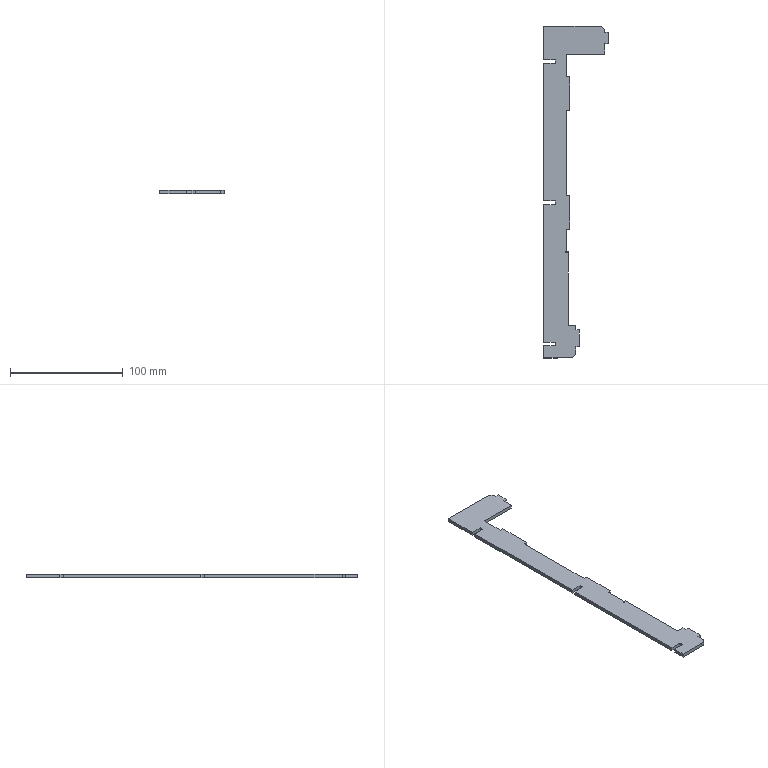Part | SolidWorks | features FlatPattern 1, SMBaseFlange 1, SheetMetal 1 | 1 solid | 46 faces | box 57 x 294.081 x 3.2 mm | volume 23149 mm3 | plane 40 | cylinder 6 | commonest cylinder face diameters 1 x2 1.5 x2 10 x2
STEP:
#1=CARTESIAN_POINT('',(397.65,-115.276,3.2));
#2=VERTEX_POINT('',#1);
#3=CARTESIAN_POINT('',(398.1,-114.588,3.2));
#4=VERTEX_POINT('',#3);
#5=CARTESIAN_POINT('',(398.4,-115.276,3.2));
#6=DIRECTION('',(0.,0.,-1.));
#7=DIRECTION('',(1.,0.,0.));
#8=AXIS2_PLACEMENT_3D('',#5,#6,#7);
#9=CIRCLE('',#8,0.75);
#10=EDGE_CURVE('',#2,#4,#9,.T.);
#11=ORIENTED_EDGE('',*,*,#10,.F.);
#12=CARTESIAN_POINT('',(397.65,-115.276,0.));
#13=VERTEX_POINT('',#12);
#14=CARTESIAN_POINT('',(397.65,-115.276,3.2));
#15=DIRECTION('',(0.,0.,-1.));
#16=VECTOR('',#15,1000.);
#17=LINE('',#14,#16);
#18=EDGE_CURVE('',#2,#13,#17,.T.);
#19=ORIENTED_EDGE('',*,*,#18,.T.);
#20=CARTESIAN_POINT('',(398.1,-114.588,0.));
#21=VERTEX_POINT('',#20);
#22=CARTESIAN_POINT('',(398.4,-115.276,0.));
#23=DIRECTION('',(0.,0.,-1.));
#24=DIRECTION('',(1.,0.,0.));
#25=AXIS2_PLACEMENT_3D('',#22,#23,#24);
#26=CIRCLE('',#25,0.75);
#27=EDGE_CURVE('',#13,#21,#26,.T.);
#28=ORIENTED_EDGE('',*,*,#27,.T.);
#29=CARTESIAN_POINT('',(398.1,-114.588,3.2));
#30=DIRECTION('',(0.,0.,-1.));
#31=VECTOR('',#30,1000.);
#32=LINE('',#29,#31);
#33=EDGE_CURVE('',#4,#21,#32,.T.);
#34=ORIENTED_EDGE('',*,*,#33,.F.);
#35=EDGE_LOOP('',(#11,#19,#28,#34));
#36=FACE_OUTER_BOUND('',#35,.T.);
#37=CARTESIAN_POINT('',(398.4,-115.276,3.2));
#38=DIRECTION('',(0.,0.,-1.));
#39=DIRECTION('',(-1.,0.,0.));
#40=AXIS2_PLACEMENT_3D('',#37,#38,#39);
#41=CYLINDRICAL_SURFACE('',#40,0.75);
#42=ADVANCED_FACE('',(#36),#41,.F.);
#43=CARTESIAN_POINT('',(432.4,59.724,0.));
#44=VERTEX_POINT('',#43);
#45=CARTESIAN_POINT('',(432.4,69.224,0.));
#46=VERTEX_POINT('',#45);
#47=CARTESIAN_POINT('',(432.4,59.724,0.));
#48=DIRECTION('',(0.,1.,0.));
#49=VECTOR('',#48,1000.);
#50=LINE('',#47,#49);
#51=EDGE_CURVE('',#44,#46,#50,.T.);
#52=ORIENTED_EDGE('',*,*,#51,.T.);
#53=CARTESIAN_POINT('',(432.4,69.224,3.2));
#54=VERTEX_POINT('',#53);
#55=CARTESIAN_POINT('',(432.4,69.224,3.2));
#56=DIRECTION('',(0.,0.,-1.));
#57=VECTOR('',#56,1000.);
#58=LINE('',#55,#57);
#59=EDGE_CURVE('',#54,#46,#58,.T.);
#60=ORIENTED_EDGE('',*,*,#59,.F.);
#61=CARTESIAN_POINT('',(432.4,59.724,3.2));
#62=VERTEX_POINT('',#61);
#63=CARTESIAN_POINT('',(432.4,59.724,3.2));
#64=DIRECTION('',(0.,1.,0.));
#65=VECTOR('',#64,1000.);
#66=LINE('',#63,#65);
#67=EDGE_CURVE('',#62,#54,#66,.T.);
#68=ORIENTED_EDGE('',*,*,#67,.F.);
#69=CARTESIAN_POINT('',(432.4,59.724,3.2));
#70=DIRECTION('',(0.,0.,-1.));
#71=VECTOR('',#70,1000.);
#72=LINE('',#69,#71);
#73=EDGE_CURVE('',#62,#44,#72,.T.);
#74=ORIENTED_EDGE('',*,*,#73,.T.);
#75=EDGE_LOOP('',(#52,#60,#68,#74));
#76=FACE_OUTER_BOUND('',#75,.T.);
#77=CARTESIAN_POINT('',(432.4,59.724,3.2));
#78=DIRECTION('',(-1.,0.,0.));
#79=DIRECTION('',(0.,0.,1.));
#80=AXIS2_PLACEMENT_3D('',#77,#78,#79);
#81=PLANE('',#80);
#82=ADVANCED_FACE('',(#76),#81,.F.);
#83=CARTESIAN_POINT('',(435.4,69.224,0.));
#84=VERTEX_POINT('',#83);
#85=CARTESIAN_POINT('',(435.4,69.224,0.));
#86=DIRECTION('',(1.,0.,0.));
#87=VECTOR('',#86,1000.);
#88=LINE('',#85,#87);
#89=EDGE_CURVE('',#46,#84,#88,.T.);
#90=ORIENTED_EDGE('',*,*,#89,.T.);
#91=CARTESIAN_POINT('',(435.4,69.224,3.2));
#92=VERTEX_POINT('',#91);
#93=CARTESIAN_POINT('',(435.4,69.224,3.2));
#94=DIRECTION('',(0.,0.,-1.));
#95=VECTOR('',#94,1000.);
#96=LINE('',#93,#95);
#97=EDGE_CURVE('',#92,#84,#96,.T.);
#98=ORIENTED_EDGE('',*,*,#97,.F.);
#99=CARTESIAN_POINT('',(435.4,69.224,3.2));
#100=DIRECTION('',(1.,0.,0.));
#101=VECTOR('',#100,1000.);
#102=LINE('',#99,#101);
#103=EDGE_CURVE('',#54,#92,#102,.T.);
#104=ORIENTED_EDGE('',*,*,#103,.F.);
#105=ORIENTED_EDGE('',*,*,#59,.T.);
#106=EDGE_LOOP('',(#90,#98,#104,#105));
#107=FACE_OUTER_BOUND('',#106,.T.);
#108=CARTESIAN_POINT('',(435.4,69.224,3.2));
#109=DIRECTION('',(0.,1.,0.));
#110=DIRECTION('',(0.,0.,1.));
#111=AXIS2_PLACEMENT_3D('',#108,#109,#110);
#112=PLANE('',#111);
#113=ADVANCED_FACE('',(#107),#112,.F.);
#114=CARTESIAN_POINT('',(435.4,79.224,0.));
#115=VERTEX_POINT('',#114);
#116=CARTESIAN_POINT('',(435.4,79.224,0.));
#117=DIRECTION('',(0.,1.,0.));
#118=VECTOR('',#117,1000.);
#119=LINE('',#116,#118);
#120=EDGE_CURVE('',#84,#115,#119,.T.);
#121=ORIENTED_EDGE('',*,*,#120,.T.);
#122=CARTESIAN_POINT('',(435.4,79.224,3.2));
#123=VERTEX_POINT('',#122);
#124=CARTESIAN_POINT('',(435.4,79.224,3.2));
#125=DIRECTION('',(0.,0.,-1.));
#126=VECTOR('',#125,1000.);
#127=LINE('',#124,#126);
#128=EDGE_CURVE('',#123,#115,#127,.T.);
#129=ORIENTED_EDGE('',*,*,#128,.F.);
#130=CARTESIAN_POINT('',(435.4,79.224,3.2));
#131=DIRECTION('',(0.,1.,0.));
#132=VECTOR('',#131,1000.);
#133=LINE('',#130,#132);
#134=EDGE_CURVE('',#92,#123,#133,.T.);
#135=ORIENTED_EDGE('',*,*,#134,.F.);
#136=ORIENTED_EDGE('',*,*,#97,.T.);
#137=EDGE_LOOP('',(#121,#129,#135,#136));
#138=FACE_OUTER_BOUND('',#137,.T.);
#139=CARTESIAN_POINT('',(435.4,79.224,3.2));
#140=DIRECTION('',(-1.,0.,0.));
#141=DIRECTION('',(0.,-1.,0.));
#142=AXIS2_PLACEMENT_3D('',#139,#140,#141);
#143=PLANE('',#142);
#144=ADVANCED_FACE('',(#138),#143,.F.);
#145=CARTESIAN_POINT('',(432.4,79.224,0.));
#146=VERTEX_POINT('',#145);
#147=CARTESIAN_POINT('',(432.4,79.224,0.));
#148=DIRECTION('',(-1.,0.,0.));
#149=VECTOR('',#148,1000.);
#150=LINE('',#147,#149);
#151=EDGE_CURVE('',#115,#146,#150,.T.);
#152=ORIENTED_EDGE('',*,*,#151,.T.);
#153=CARTESIAN_POINT('',(432.4,79.224,3.2));
#154=VERTEX_POINT('',#153);
#155=CARTESIAN_POINT('',(432.4,79.224,3.2));
#156=DIRECTION('',(0.,0.,-1.));
#157=VECTOR('',#156,1000.);
#158=LINE('',#155,#157);
#159=EDGE_CURVE('',#154,#146,#158,.T.);
#160=ORIENTED_EDGE('',*,*,#159,.F.);
#161=CARTESIAN_POINT('',(432.4,79.224,3.2));
#162=DIRECTION('',(-1.,0.,0.));
#163=VECTOR('',#162,1000.);
#164=LINE('',#161,#163);
#165=EDGE_CURVE('',#123,#154,#164,.T.);
#166=ORIENTED_EDGE('',*,*,#165,.F.);
#167=ORIENTED_EDGE('',*,*,#128,.T.);
#168=EDGE_LOOP('',(#152,#160,#166,#167));
#169=FACE_OUTER_BOUND('',#168,.T.);
#170=CARTESIAN_POINT('',(432.4,79.224,3.2));
#171=DIRECTION('',(0.,-1.,0.));
#172=DIRECTION('',(1.,0.,0.));
#173=AXIS2_PLACEMENT_3D('',#170,#171,#172);
#174=PLANE('',#173);
#175=ADVANCED_FACE('',(#169),#174,.F.);
#176=CARTESIAN_POINT('',(432.4,79.724,0.));
#177=VERTEX_POINT('',#176);
#178=CARTESIAN_POINT('',(432.4,79.224,0.));
#179=DIRECTION('',(0.,1.,0.));
#180=VECTOR('',#179,1000.);
#181=LINE('',#178,#180);
#182=EDGE_CURVE('',#146,#177,#181,.T.);
#183=ORIENTED_EDGE('',*,*,#182,.T.);
#184=CARTESIAN_POINT('',(432.4,79.724,3.2));
#185=VERTEX_POINT('',#184);
#186=CARTESIAN_POINT('',(432.4,79.724,3.2));
#187=DIRECTION('',(0.,0.,-1.));
#188=VECTOR('',#187,1000.);
#189=LINE('',#186,#188);
#190=EDGE_CURVE('',#185,#177,#189,.T.);
#191=ORIENTED_EDGE('',*,*,#190,.F.);
#192=CARTESIAN_POINT('',(432.4,79.224,3.2));
#193=DIRECTION('',(0.,1.,0.));
#194=VECTOR('',#193,1000.);
#195=LINE('',#192,#194);
#196=EDGE_CURVE('',#154,#185,#195,.T.);
#197=ORIENTED_EDGE('',*,*,#196,.F.);
#198=ORIENTED_EDGE('',*,*,#159,.T.);
#199=EDGE_LOOP('',(#183,#191,#197,#198));
#200=FACE_OUTER_BOUND('',#199,.T.);
#201=CARTESIAN_POINT('',(432.4,79.224,3.2));
#202=DIRECTION('',(-1.,0.,0.));
#203=DIRECTION('',(0.,0.,1.));
#204=AXIS2_PLACEMENT_3D('',#201,#202,#203);
#205=PLANE('',#204);
#206=ADVANCED_FACE('',(#200),#205,.F.);
#207=CARTESIAN_POINT('',(427.4,84.724,0.));
#208=VERTEX_POINT('',#207);
#209=CARTESIAN_POINT('',(427.4,79.724,0.));
#210=DIRECTION('',(0.,0.,1.));
#211=DIRECTION('',(-1.,0.,0.));
#212=AXIS2_PLACEMENT_3D('',#209,#210,#211);
#213=CIRCLE('',#212,5.);
#214=EDGE_CURVE('',#177,#208,#213,.T.);
#215=ORIENTED_EDGE('',*,*,#214,.T.);
#216=CARTESIAN_POINT('',(427.4,84.724,3.2));
#217=VERTEX_POINT('',#216);
#218=CARTESIAN_POINT('',(427.4,84.724,3.2));
#219=DIRECTION('',(0.,0.,-1.));
#220=VECTOR('',#219,1000.);
#221=LINE('',#218,#220);
#222=EDGE_CURVE('',#217,#208,#221,.T.);
#223=ORIENTED_EDGE('',*,*,#222,.F.);
#224=CARTESIAN_POINT('',(427.4,79.724,3.2));
#225=DIRECTION('',(0.,0.,1.));
#226=DIRECTION('',(-1.,0.,0.));
#227=AXIS2_PLACEMENT_3D('',#224,#225,#226);
#228=CIRCLE('',#227,5.);
#229=EDGE_CURVE('',#185,#217,#228,.T.);
#230=ORIENTED_EDGE('',*,*,#229,.F.);
#231=ORIENTED_EDGE('',*,*,#190,.T.);
#232=EDGE_LOOP('',(#215,#223,#230,#231));
#233=FACE_OUTER_BOUND('',#232,.T.);
#234=CARTESIAN_POINT('',(427.4,79.724,3.2));
#235=DIRECTION('',(0.,0.,-1.));
#236=DIRECTION('',(-1.,0.,0.));
#237=AXIS2_PLACEMENT_3D('',#234,#235,#236);
#238=CYLINDRICAL_SURFACE('',#237,5.);
#239=ADVANCED_FACE('',(#233),#238,.T.);
#240=CARTESIAN_POINT('',(378.4,84.724,0.));
#241=VERTEX_POINT('',#240);
#242=CARTESIAN_POINT('',(427.4,84.724,0.));
#243=DIRECTION('',(-1.,0.,0.));
#244=VECTOR('',#243,1000.);
#245=LINE('',#242,#244);
#246=EDGE_CURVE('',#208,#241,#245,.T.);
#247=ORIENTED_EDGE('',*,*,#246,.T.);
#248=CARTESIAN_POINT('',(378.4,84.724,3.2));
#249=VERTEX_POINT('',#248);
#250=CARTESIAN_POINT('',(378.4,84.724,3.2));
#251=DIRECTION('',(0.,0.,-1.));
#252=VECTOR('',#251,1000.);
#253=LINE('',#250,#252);
#254=EDGE_CURVE('',#249,#241,#253,.T.);
#255=ORIENTED_EDGE('',*,*,#254,.F.);
#256=CARTESIAN_POINT('',(427.4,84.724,3.2));
#257=DIRECTION('',(-1.,0.,0.));
#258=VECTOR('',#257,1000.);
#259=LINE('',#256,#258);
#260=EDGE_CURVE('',#217,#249,#259,.T.);
#261=ORIENTED_EDGE('',*,*,#260,.F.);
#262=ORIENTED_EDGE('',*,*,#222,.T.);
#263=EDGE_LOOP('',(#247,#255,#261,#262));
#264=FACE_OUTER_BOUND('',#263,.T.);
#265=CARTESIAN_POINT('',(427.4,84.724,3.2));
#266=DIRECTION('',(0.,-1.,0.));
#267=DIRECTION('',(1.,0.,0.));
#268=AXIS2_PLACEMENT_3D('',#265,#266,#267);
#269=PLANE('',#268);
#270=ADVANCED_FACE('',(#264),#269,.F.);
#271=CARTESIAN_POINT('',(378.4,54.724,0.));
#272=VERTEX_POINT('',#271);
#273=CARTESIAN_POINT('',(378.4,84.724,0.));
#274=DIRECTION('',(0.,-1.,0.));
#275=VECTOR('',#274,1000.);
#276=LINE('',#273,#275);
#277=EDGE_CURVE('',#241,#272,#276,.T.);
#278=ORIENTED_EDGE('',*,*,#277,.T.);
#279=CARTESIAN_POINT('',(378.4,54.724,3.2));
#280=VERTEX_POINT('',#279);
#281=CARTESIAN_POINT('',(378.4,54.724,3.2));
#282=DIRECTION('',(0.,0.,-1.));
#283=VECTOR('',#282,1000.);
#284=LINE('',#281,#283);
#285=EDGE_CURVE('',#280,#272,#284,.T.);
#286=ORIENTED_EDGE('',*,*,#285,.F.);
#287=CARTESIAN_POINT('',(378.4,84.724,3.2));
#288=DIRECTION('',(0.,-1.,0.));
#289=VECTOR('',#288,1000.);
#290=LINE('',#287,#289);
#291=EDGE_CURVE('',#249,#280,#290,.T.);
#292=ORIENTED_EDGE('',*,*,#291,.F.);
#293=ORIENTED_EDGE('',*,*,#254,.T.);
#294=EDGE_LOOP('',(#278,#286,#292,#293));
#295=FACE_OUTER_BOUND('',#294,.T.);
#296=CARTESIAN_POINT('',(378.4,84.724,3.2));
#297=DIRECTION('',(1.,0.,0.));
#298=DIRECTION('',(0.,1.,0.));
#299=AXIS2_PLACEMENT_3D('',#296,#297,#298);
#300=PLANE('',#299);
#301=ADVANCED_FACE('',(#295),#300,.F.);
#302=CARTESIAN_POINT('',(388.4,54.724,0.));
#303=VERTEX_POINT('',#302);
#304=CARTESIAN_POINT('',(378.4,54.724,0.));
#305=DIRECTION('',(1.,0.000000036,0.));
#306=VECTOR('',#305,1000.);
#307=LINE('',#304,#306);
#308=EDGE_CURVE('',#272,#303,#307,.T.);
#309=ORIENTED_EDGE('',*,*,#308,.T.);
#310=CARTESIAN_POINT('',(388.4,54.724,3.2));
#311=VERTEX_POINT('',#310);
#312=CARTESIAN_POINT('',(388.4,54.724,3.2));
#313=DIRECTION('',(0.,0.,-1.));
#314=VECTOR('',#313,1000.);
#315=LINE('',#312,#314);
#316=EDGE_CURVE('',#311,#303,#315,.T.);
#317=ORIENTED_EDGE('',*,*,#316,.F.);
#318=CARTESIAN_POINT('',(378.4,54.724,3.2));
#319=DIRECTION('',(1.,0.000000036,0.));
#320=VECTOR('',#319,1000.);
#321=LINE('',#318,#320);
#322=EDGE_CURVE('',#280,#311,#321,.T.);
#323=ORIENTED_EDGE('',*,*,#322,.F.);
#324=ORIENTED_EDGE('',*,*,#285,.T.);
#325=EDGE_LOOP('',(#309,#317,#323,#324));
#326=FACE_OUTER_BOUND('',#325,.T.);
#327=CARTESIAN_POINT('',(378.4,54.724,3.2));
#328=DIRECTION('',(-0.000000036,1.,0.));
#329=DIRECTION('',(-1.,-0.000000036,0.));
#330=AXIS2_PLACEMENT_3D('',#327,#328,#329);
#331=PLANE('',#330);
#332=ADVANCED_FACE('',(#326),#331,.F.);
#333=CARTESIAN_POINT('',(388.4,51.524,0.));
#334=VERTEX_POINT('',#333);
#335=CARTESIAN_POINT('',(388.4,54.724,0.));
#336=DIRECTION('',(0.,-1.,0.));
#337=VECTOR('',#336,1000.);
#338=LINE('',#335,#337);
#339=EDGE_CURVE('',#303,#334,#338,.T.);
#340=ORIENTED_EDGE('',*,*,#339,.T.);
#341=CARTESIAN_POINT('',(388.4,51.524,3.2));
#342=VERTEX_POINT('',#341);
#343=CARTESIAN_POINT('',(388.4,51.524,3.2));
#344=DIRECTION('',(0.,0.,-1.));
#345=VECTOR('',#344,1000.);
#346=LINE('',#343,#345);
#347=EDGE_CURVE('',#342,#334,#346,.T.);
#348=ORIENTED_EDGE('',*,*,#347,.F.);
#349=CARTESIAN_POINT('',(388.4,54.724,3.2));
#350=DIRECTION('',(0.,-1.,0.));
#351=VECTOR('',#350,1000.);
#352=LINE('',#349,#351);
#353=EDGE_CURVE('',#311,#342,#352,.T.);
#354=ORIENTED_EDGE('',*,*,#353,.F.);
#355=ORIENTED_EDGE('',*,*,#316,.T.);
#356=EDGE_LOOP('',(#340,#348,#354,#355));
#357=FACE_OUTER_BOUND('',#356,.T.);
#358=CARTESIAN_POINT('',(388.4,54.724,3.2));
#359=DIRECTION('',(1.,0.,0.));
#360=DIRECTION('',(0.,0.,-1.));
#361=AXIS2_PLACEMENT_3D('',#358,#359,#360);
#362=PLANE('',#361);
#363=ADVANCED_FACE('',(#357),#362,.F.);
#364=CARTESIAN_POINT('',(378.4,51.524,0.));
#365=VERTEX_POINT('',#364);
#366=CARTESIAN_POINT('',(388.4,51.524,0.));
#367=DIRECTION('',(-1.,-0.000000036,0.));
#368=VECTOR('',#367,1000.);
#369=LINE('',#366,#368);
#370=EDGE_CURVE('',#334,#365,#369,.T.);
#371=ORIENTED_EDGE('',*,*,#370,.T.);
#372=CARTESIAN_POINT('',(378.4,51.524,3.2));
#373=VERTEX_POINT('',#372);
#374=CARTESIAN_POINT('',(378.4,51.524,3.2));
#375=DIRECTION('',(0.,0.,-1.));
#376=VECTOR('',#375,1000.);
#377=LINE('',#374,#376);
#378=EDGE_CURVE('',#373,#365,#377,.T.);
#379=ORIENTED_EDGE('',*,*,#378,.F.);
#380=CARTESIAN_POINT('',(388.4,51.524,3.2));
#381=DIRECTION('',(-1.,-0.000000036,0.));
#382=VECTOR('',#381,1000.);
#383=LINE('',#380,#382);
#384=EDGE_CURVE('',#342,#373,#383,.T.);
#385=ORIENTED_EDGE('',*,*,#384,.F.);
#386=ORIENTED_EDGE('',*,*,#347,.T.);
#387=EDGE_LOOP('',(#371,#379,#385,#386));
#388=FACE_OUTER_BOUND('',#387,.T.);
#389=CARTESIAN_POINT('',(388.4,51.524,3.2));
#390=DIRECTION('',(0.000000036,-1.,0.));
#391=DIRECTION('',(1.,0.000000036,0.));
#392=AXIS2_PLACEMENT_3D('',#389,#390,#391);
#393=PLANE('',#392);
#394=ADVANCED_FACE('',(#388),#393,.F.);
#395=CARTESIAN_POINT('',(378.4,-70.276,0.));
#396=VERTEX_POINT('',#395);
#397=CARTESIAN_POINT('',(378.4,51.524,0.));
#398=DIRECTION('',(0.,-1.,0.));
#399=VECTOR('',#398,1000.);
#400=LINE('',#397,#399);
#401=EDGE_CURVE('',#365,#396,#400,.T.);
#402=ORIENTED_EDGE('',*,*,#401,.T.);
#403=CARTESIAN_POINT('',(378.4,-70.276,3.2));
#404=VERTEX_POINT('',#403);
#405=CARTESIAN_POINT('',(378.4,-70.276,3.2));
#406=DIRECTION('',(0.,0.,-1.));
#407=VECTOR('',#406,1000.);
#408=LINE('',#405,#407);
#409=EDGE_CURVE('',#404,#396,#408,.T.);
#410=ORIENTED_EDGE('',*,*,#409,.F.);
#411=CARTESIAN_POINT('',(378.4,51.524,3.2));
#412=DIRECTION('',(0.,-1.,0.));
#413=VECTOR('',#412,1000.);
#414=LINE('',#411,#413);
#415=EDGE_CURVE('',#373,#404,#414,.T.);
#416=ORIENTED_EDGE('',*,*,#415,.F.);
#417=ORIENTED_EDGE('',*,*,#378,.T.);
#418=EDGE_LOOP('',(#402,#410,#416,#417));
#419=FACE_OUTER_BOUND('',#418,.T.);
#420=CARTESIAN_POINT('',(378.4,51.524,3.2));
#421=DIRECTION('',(1.,0.,0.));
#422=DIRECTION('',(0.,0.,-1.));
#423=AXIS2_PLACEMENT_3D('',#420,#421,#422);
#424=PLANE('',#423);
#425=ADVANCED_FACE('',(#419),#424,.F.);
#426=CARTESIAN_POINT('',(388.4,-70.276,0.));
#427=VERTEX_POINT('',#426);
#428=CARTESIAN_POINT('',(378.4,-70.276,0.));
#429=DIRECTION('',(1.,0.000000036,0.));
#430=VECTOR('',#429,1000.);
#431=LINE('',#428,#430);
#432=EDGE_CURVE('',#396,#427,#431,.T.);
#433=ORIENTED_EDGE('',*,*,#432,.T.);
#434=CARTESIAN_POINT('',(388.4,-70.276,3.2));
#435=VERTEX_POINT('',#434);
#436=CARTESIAN_POINT('',(388.4,-70.276,3.2));
#437=DIRECTION('',(0.,0.,-1.));
#438=VECTOR('',#437,1000.);
#439=LINE('',#436,#438);
#440=EDGE_CURVE('',#435,#427,#439,.T.);
#441=ORIENTED_EDGE('',*,*,#440,.F.);
#442=CARTESIAN_POINT('',(378.4,-70.276,3.2));
#443=DIRECTION('',(1.,0.000000036,0.));
#444=VECTOR('',#443,1000.);
#445=LINE('',#442,#444);
#446=EDGE_CURVE('',#404,#435,#445,.T.);
#447=ORIENTED_EDGE('',*,*,#446,.F.);
#448=ORIENTED_EDGE('',*,*,#409,.T.);
#449=EDGE_LOOP('',(#433,#441,#447,#448));
#450=FACE_OUTER_BOUND('',#449,.T.);
#451=CARTESIAN_POINT('',(378.4,-70.276,3.2));
#452=DIRECTION('',(-0.000000036,1.,0.));
#453=DIRECTION('',(-1.,-0.000000036,0.));
#454=AXIS2_PLACEMENT_3D('',#451,#452,#453);
#455=PLANE('',#454);
#456=ADVANCED_FACE('',(#450),#455,.F.);
#457=CARTESIAN_POINT('',(388.4,-73.476,0.));
#458=VERTEX_POINT('',#457);
#459=CARTESIAN_POINT('',(388.4,-70.276,0.));
#460=DIRECTION('',(0.,-1.,0.));
#461=VECTOR('',#460,1000.);
#462=LINE('',#459,#461);
#463=EDGE_CURVE('',#427,#458,#462,.T.);
#464=ORIENTED_EDGE('',*,*,#463,.T.);
#465=CARTESIAN_POINT('',(388.4,-73.476,3.2));
#466=VERTEX_POINT('',#465);
#467=CARTESIAN_POINT('',(388.4,-73.476,3.2));
#468=DIRECTION('',(0.,0.,-1.));
#469=VECTOR('',#468,1000.);
#470=LINE('',#467,#469);
#471=EDGE_CURVE('',#466,#458,#470,.T.);
#472=ORIENTED_EDGE('',*,*,#471,.F.);
#473=CARTESIAN_POINT('',(388.4,-70.276,3.2));
#474=DIRECTION('',(0.,-1.,0.));
#475=VECTOR('',#474,1000.);
#476=LINE('',#473,#475);
#477=EDGE_CURVE('',#435,#466,#476,.T.);
#478=ORIENTED_EDGE('',*,*,#477,.F.);
#479=ORIENTED_EDGE('',*,*,#440,.T.);
#480=EDGE_LOOP('',(#464,#472,#478,#479));
#481=FACE_OUTER_BOUND('',#480,.T.);
#482=CARTESIAN_POINT('',(388.4,-70.276,3.2));
#483=DIRECTION('',(1.,0.,0.));
#484=DIRECTION('',(0.,0.,-1.));
#485=AXIS2_PLACEMENT_3D('',#482,#483,#484);
#486=PLANE('',#485);
#487=ADVANCED_FACE('',(#481),#486,.F.);
#488=CARTESIAN_POINT('',(378.4,-73.476,0.));
#489=VERTEX_POINT('',#488);
#490=CARTESIAN_POINT('',(388.4,-73.476,0.));
#491=DIRECTION('',(-1.,0.,0.));
#492=VECTOR('',#491,1000.);
#493=LINE('',#490,#492);
#494=EDGE_CURVE('',#458,#489,#493,.T.);
#495=ORIENTED_EDGE('',*,*,#494,.T.);
#496=CARTESIAN_POINT('',(378.4,-73.476,3.2));
#497=VERTEX_POINT('',#496);
#498=CARTESIAN_POINT('',(378.4,-73.476,3.2));
#499=DIRECTION('',(0.,0.,-1.));
#500=VECTOR('',#499,1000.);
#501=LINE('',#498,#500);
#502=EDGE_CURVE('',#497,#489,#501,.T.);
#503=ORIENTED_EDGE('',*,*,#502,.F.);
#504=CARTESIAN_POINT('',(388.4,-73.476,3.2));
#505=DIRECTION('',(-1.,0.,0.));
#506=VECTOR('',#505,1000.);
#507=LINE('',#504,#506);
#508=EDGE_CURVE('',#466,#497,#507,.T.);
#509=ORIENTED_EDGE('',*,*,#508,.F.);
#510=ORIENTED_EDGE('',*,*,#471,.T.);
#511=EDGE_LOOP('',(#495,#503,#509,#510));
#512=FACE_OUTER_BOUND('',#511,.T.);
#513=CARTESIAN_POINT('',(388.4,-73.476,3.2));
#514=DIRECTION('',(0.,-1.,0.));
#515=DIRECTION('',(0.,0.,-1.));
#516=AXIS2_PLACEMENT_3D('',#513,#514,#515);
#517=PLANE('',#516);
#518=ADVANCED_FACE('',(#512),#517,.F.);
#519=CARTESIAN_POINT('',(378.4,-195.276,0.));
#520=VERTEX_POINT('',#519);
#521=CARTESIAN_POINT('',(378.4,-73.476,0.));
#522=DIRECTION('',(0.,-1.,0.));
#523=VECTOR('',#522,1000.);
#524=LINE('',#521,#523);
#525=EDGE_CURVE('',#489,#520,#524,.T.);
#526=ORIENTED_EDGE('',*,*,#525,.T.);
#527=CARTESIAN_POINT('',(378.4,-195.276,3.2));
#528=VERTEX_POINT('',#527);
#529=CARTESIAN_POINT('',(378.4,-195.276,3.2));
#530=DIRECTION('',(0.,0.,-1.));
#531=VECTOR('',#530,1000.);
#532=LINE('',#529,#531);
#533=EDGE_CURVE('',#528,#520,#532,.T.);
#534=ORIENTED_EDGE('',*,*,#533,.F.);
#535=CARTESIAN_POINT('',(378.4,-73.476,3.2));
#536=DIRECTION('',(0.,-1.,0.));
#537=VECTOR('',#536,1000.);
#538=LINE('',#535,#537);
#539=EDGE_CURVE('',#497,#528,#538,.T.);
#540=ORIENTED_EDGE('',*,*,#539,.F.);
#541=ORIENTED_EDGE('',*,*,#502,.T.);
#542=EDGE_LOOP('',(#526,#534,#540,#541));
#543=FACE_OUTER_BOUND('',#542,.T.);
#544=CARTESIAN_POINT('',(378.4,-73.476,3.2));
#545=DIRECTION('',(1.,0.,0.));
#546=DIRECTION('',(0.,0.,-1.));
#547=AXIS2_PLACEMENT_3D('',#544,#545,#546);
#548=PLANE('',#547);
#549=ADVANCED_FACE('',(#543),#548,.F.);
#550=CARTESIAN_POINT('',(388.4,-195.276,0.));
#551=VERTEX_POINT('',#550);
#552=CARTESIAN_POINT('',(378.4,-195.276,0.));
#553=DIRECTION('',(1.,0.000000072,0.));
#554=VECTOR('',#553,1000.);
#555=LINE('',#552,#554);
#556=EDGE_CURVE('',#520,#551,#555,.T.);
#557=ORIENTED_EDGE('',*,*,#556,.T.);
#558=CARTESIAN_POINT('',(388.4,-195.276,3.2));
#559=VERTEX_POINT('',#558);
#560=CARTESIAN_POINT('',(388.4,-195.276,3.2));
#561=DIRECTION('',(0.,0.,-1.));
#562=VECTOR('',#561,1000.);
#563=LINE('',#560,#562);
#564=EDGE_CURVE('',#559,#551,#563,.T.);
#565=ORIENTED_EDGE('',*,*,#564,.F.);
#566=CARTESIAN_POINT('',(378.4,-195.276,3.2));
#567=DIRECTION('',(1.,0.000000072,0.));
#568=VECTOR('',#567,1000.);
#569=LINE('',#566,#568);
#570=EDGE_CURVE('',#528,#559,#569,.T.);
#571=ORIENTED_EDGE('',*,*,#570,.F.);
#572=ORIENTED_EDGE('',*,*,#533,.T.);
#573=EDGE_LOOP('',(#557,#565,#571,#572));
#574=FACE_OUTER_BOUND('',#573,.T.);
#575=CARTESIAN_POINT('',(378.4,-195.276,3.2));
#576=DIRECTION('',(-0.000000072,1.,0.));
#577=DIRECTION('',(-1.,-0.000000072,0.));
#578=AXIS2_PLACEMENT_3D('',#575,#576,#577);
#579=PLANE('',#578);
#580=ADVANCED_FACE('',(#574),#579,.F.);
#581=CARTESIAN_POINT('',(388.4,-198.476,0.));
#582=VERTEX_POINT('',#581);
#583=CARTESIAN_POINT('',(388.4,-195.276,0.));
#584=DIRECTION('',(0.,-1.,0.));
#585=VECTOR('',#584,1000.);
#586=LINE('',#583,#585);
#587=EDGE_CURVE('',#551,#582,#586,.T.);
#588=ORIENTED_EDGE('',*,*,#587,.T.);
#589=CARTESIAN_POINT('',(388.4,-198.476,3.2));
#590=VERTEX_POINT('',#589);
#591=CARTESIAN_POINT('',(388.4,-198.476,3.2));
#592=DIRECTION('',(0.,0.,-1.));
#593=VECTOR('',#592,1000.);
#594=LINE('',#591,#593);
#595=EDGE_CURVE('',#590,#582,#594,.T.);
#596=ORIENTED_EDGE('',*,*,#595,.F.);
#597=CARTESIAN_POINT('',(388.4,-195.276,3.2));
#598=DIRECTION('',(0.,-1.,0.));
#599=VECTOR('',#598,1000.);
#600=LINE('',#597,#599);
#601=EDGE_CURVE('',#559,#590,#600,.T.);
#602=ORIENTED_EDGE('',*,*,#601,.F.);
#603=ORIENTED_EDGE('',*,*,#564,.T.);
#604=EDGE_LOOP('',(#588,#596,#602,#603));
#605=FACE_OUTER_BOUND('',#604,.T.);
#606=CARTESIAN_POINT('',(388.4,-195.276,3.2));
#607=DIRECTION('',(1.,0.,0.));
#608=DIRECTION('',(0.,0.,-1.));
#609=AXIS2_PLACEMENT_3D('',#606,#607,#608);
#610=PLANE('',#609);
#611=ADVANCED_FACE('',(#605),#610,.F.);
#612=CARTESIAN_POINT('',(378.4,-198.476,0.));
#613=VERTEX_POINT('',#612);
#614=CARTESIAN_POINT('',(388.4,-198.476,0.));
#615=DIRECTION('',(-1.,-0.000000036,0.));
#616=VECTOR('',#615,1000.);
#617=LINE('',#614,#616);
#618=EDGE_CURVE('',#582,#613,#617,.T.);
#619=ORIENTED_EDGE('',*,*,#618,.T.);
#620=CARTESIAN_POINT('',(378.4,-198.476,3.2));
#621=VERTEX_POINT('',#620);
#622=CARTESIAN_POINT('',(378.4,-198.476,3.2));
#623=DIRECTION('',(0.,0.,-1.));
#624=VECTOR('',#623,1000.);
#625=LINE('',#622,#624);
#626=EDGE_CURVE('',#621,#613,#625,.T.);
#627=ORIENTED_EDGE('',*,*,#626,.F.);
#628=CARTESIAN_POINT('',(388.4,-198.476,3.2));
#629=DIRECTION('',(-1.,-0.000000036,0.));
#630=VECTOR('',#629,1000.);
#631=LINE('',#628,#630);
#632=EDGE_CURVE('',#590,#621,#631,.T.);
#633=ORIENTED_EDGE('',*,*,#632,.F.);
#634=ORIENTED_EDGE('',*,*,#595,.T.);
#635=EDGE_LOOP('',(#619,#627,#633,#634));
#636=FACE_OUTER_BOUND('',#635,.T.);
#637=CARTESIAN_POINT('',(388.4,-198.476,3.2));
#638=DIRECTION('',(0.000000036,-1.,0.));
#639=DIRECTION('',(1.,0.000000036,0.));
#640=AXIS2_PLACEMENT_3D('',#637,#638,#639);
#641=PLANE('',#640);
#642=ADVANCED_FACE('',(#636),#641,.F.);
#643=CARTESIAN_POINT('',(378.4,-209.357,0.));
#644=VERTEX_POINT('',#643);
#645=CARTESIAN_POINT('',(378.4,-198.476,0.));
#646=DIRECTION('',(0.,-1.,0.));
#647=VECTOR('',#646,1000.);
#648=LINE('',#645,#647);
#649=EDGE_CURVE('',#613,#644,#648,.T.);
#650=ORIENTED_EDGE('',*,*,#649,.T.);
#651=CARTESIAN_POINT('',(378.4,-209.357,3.2));
#652=VERTEX_POINT('',#651);
#653=CARTESIAN_POINT('',(378.4,-209.357,3.2));
#654=DIRECTION('',(0.,0.,-1.));
#655=VECTOR('',#654,1000.);
#656=LINE('',#653,#655);
#657=EDGE_CURVE('',#652,#644,#656,.T.);
#658=ORIENTED_EDGE('',*,*,#657,.F.);
#659=CARTESIAN_POINT('',(378.4,-198.476,3.2));
#660=DIRECTION('',(0.,-1.,0.));
#661=VECTOR('',#660,1000.);
#662=LINE('',#659,#661);
#663=EDGE_CURVE('',#621,#652,#662,.T.);
#664=ORIENTED_EDGE('',*,*,#663,.F.);
#665=ORIENTED_EDGE('',*,*,#626,.T.);
#666=EDGE_LOOP('',(#650,#658,#664,#665));
#667=FACE_OUTER_BOUND('',#666,.T.);
#668=CARTESIAN_POINT('',(378.4,-198.476,3.2));
#669=DIRECTION('',(1.,0.,0.));
#670=DIRECTION('',(0.,0.,-1.));
#671=AXIS2_PLACEMENT_3D('',#668,#669,#670);
#672=PLANE('',#671);
#673=ADVANCED_FACE('',(#667),#672,.F.);
#674=CARTESIAN_POINT('',(401.9,-209.357,0.));
#675=VERTEX_POINT('',#674);
#676=CARTESIAN_POINT('',(378.4,-209.357,0.));
#677=DIRECTION('',(1.,0.,0.));
#678=VECTOR('',#677,1000.);
#679=LINE('',#676,#678);
#680=EDGE_CURVE('',#644,#675,#679,.T.);
#681=ORIENTED_EDGE('',*,*,#680,.T.);
#682=CARTESIAN_POINT('',(401.9,-209.357,3.2));
#683=VERTEX_POINT('',#682);
#684=CARTESIAN_POINT('',(401.9,-209.357,3.2));
#685=DIRECTION('',(0.,0.,-1.));
#686=VECTOR('',#685,1000.);
#687=LINE('',#684,#686);
#688=EDGE_CURVE('',#683,#675,#687,.T.);
#689=ORIENTED_EDGE('',*,*,#688,.F.);
#690=CARTESIAN_POINT('',(378.4,-209.357,3.2));
#691=DIRECTION('',(1.,0.,0.));
#692=VECTOR('',#691,1000.);
#693=LINE('',#690,#692);
#694=EDGE_CURVE('',#652,#683,#693,.T.);
#695=ORIENTED_EDGE('',*,*,#694,.F.);
#696=ORIENTED_EDGE('',*,*,#657,.T.);
#697=EDGE_LOOP('',(#681,#689,#695,#696));
#698=FACE_OUTER_BOUND('',#697,.T.);
#699=CARTESIAN_POINT('',(378.4,-209.357,3.2));
#700=DIRECTION('',(0.,1.,0.));
#701=DIRECTION('',(0.,0.,1.));
#702=AXIS2_PLACEMENT_3D('',#699,#700,#701);
#703=PLANE('',#702);
#704=ADVANCED_FACE('',(#698),#703,.F.);
#705=CARTESIAN_POINT('',(406.9,-204.357,0.));
#706=VERTEX_POINT('',#705);
#707=CARTESIAN_POINT('',(401.9,-204.357,0.));
#708=DIRECTION('',(0.,0.,1.));
#709=DIRECTION('',(1.,0.,0.));
#710=AXIS2_PLACEMENT_3D('',#707,#708,#709);
#711=CIRCLE('',#710,5.);
#712=EDGE_CURVE('',#675,#706,#711,.T.);
#713=ORIENTED_EDGE('',*,*,#712,.T.);
#714=CARTESIAN_POINT('',(406.9,-204.357,3.2));
#715=VERTEX_POINT('',#714);
#716=CARTESIAN_POINT('',(406.9,-204.357,3.2));
#717=DIRECTION('',(0.,0.,-1.));
#718=VECTOR('',#717,1000.);
#719=LINE('',#716,#718);
#720=EDGE_CURVE('',#715,#706,#719,.T.);
#721=ORIENTED_EDGE('',*,*,#720,.F.);
#722=CARTESIAN_POINT('',(401.9,-204.357,3.2));
#723=DIRECTION('',(0.,0.,1.));
#724=DIRECTION('',(1.,0.,0.));
#725=AXIS2_PLACEMENT_3D('',#722,#723,#724);
#726=CIRCLE('',#725,5.);
#727=EDGE_CURVE('',#683,#715,#726,.T.);
#728=ORIENTED_EDGE('',*,*,#727,.F.);
#729=ORIENTED_EDGE('',*,*,#688,.T.);
#730=EDGE_LOOP('',(#713,#721,#728,#729));
#731=FACE_OUTER_BOUND('',#730,.T.);
#732=CARTESIAN_POINT('',(401.9,-204.357,3.2));
#733=DIRECTION('',(0.,0.,-1.));
#734=DIRECTION('',(-1.,0.,0.));
#735=AXIS2_PLACEMENT_3D('',#732,#733,#734);
#736=CYLINDRICAL_SURFACE('',#735,5.);
#737=ADVANCED_FACE('',(#731),#736,.T.);
#738=CARTESIAN_POINT('',(406.9,-199.357,0.));
#739=VERTEX_POINT('',#738);
#740=CARTESIAN_POINT('',(406.9,-204.357,0.));
#741=DIRECTION('',(0.,1.,0.));
#742=VECTOR('',#741,1000.);
#743=LINE('',#740,#742);
#744=EDGE_CURVE('',#706,#739,#743,.T.);
#745=ORIENTED_EDGE('',*,*,#744,.T.);
#746=CARTESIAN_POINT('',(406.9,-199.357,3.2));
#747=VERTEX_POINT('',#746);
#748=CARTESIAN_POINT('',(406.9,-199.357,3.2));
#749=DIRECTION('',(0.,0.,-1.));
#750=VECTOR('',#749,1000.);
#751=LINE('',#748,#750);
#752=EDGE_CURVE('',#747,#739,#751,.T.);
#753=ORIENTED_EDGE('',*,*,#752,.F.);
#754=CARTESIAN_POINT('',(406.9,-204.357,3.2));
#755=DIRECTION('',(0.,1.,0.));
#756=VECTOR('',#755,1000.);
#757=LINE('',#754,#756);
#758=EDGE_CURVE('',#715,#747,#757,.T.);
#759=ORIENTED_EDGE('',*,*,#758,.F.);
#760=ORIENTED_EDGE('',*,*,#720,.T.);
#761=EDGE_LOOP('',(#745,#753,#759,#760));
#762=FACE_OUTER_BOUND('',#761,.T.);
#763=CARTESIAN_POINT('',(406.9,-204.357,3.2));
#764=DIRECTION('',(-1.,0.,0.));
#765=DIRECTION('',(0.,-1.,0.));
#766=AXIS2_PLACEMENT_3D('',#763,#764,#765);
#767=PLANE('',#766);
#768=ADVANCED_FACE('',(#762),#767,.F.);
#769=CARTESIAN_POINT('',(409.9,-199.357,0.));
#770=VERTEX_POINT('',#769);
#771=CARTESIAN_POINT('',(406.9,-199.357,0.));
#772=DIRECTION('',(1.,0.,0.));
#773=VECTOR('',#772,1000.);
#774=LINE('',#771,#773);
#775=EDGE_CURVE('',#739,#770,#774,.T.);
#776=ORIENTED_EDGE('',*,*,#775,.T.);
#777=CARTESIAN_POINT('',(409.9,-199.357,3.2));
#778=VERTEX_POINT('',#777);
#779=CARTESIAN_POINT('',(409.9,-199.357,3.2));
#780=DIRECTION('',(0.,0.,-1.));
#781=VECTOR('',#780,1000.);
#782=LINE('',#779,#781);
#783=EDGE_CURVE('',#778,#770,#782,.T.);
#784=ORIENTED_EDGE('',*,*,#783,.F.);
#785=CARTESIAN_POINT('',(406.9,-199.357,3.2));
#786=DIRECTION('',(1.,0.,0.));
#787=VECTOR('',#786,1000.);
#788=LINE('',#785,#787);
#789=EDGE_CURVE('',#747,#778,#788,.T.);
#790=ORIENTED_EDGE('',*,*,#789,.F.);
#791=ORIENTED_EDGE('',*,*,#752,.T.);
#792=EDGE_LOOP('',(#776,#784,#790,#791));
#793=FACE_OUTER_BOUND('',#792,.T.);
#794=CARTESIAN_POINT('',(406.9,-199.357,3.2));
#795=DIRECTION('',(0.,1.,0.));
#796=DIRECTION('',(0.,0.,1.));
#797=AXIS2_PLACEMENT_3D('',#794,#795,#796);
#798=PLANE('',#797);
#799=ADVANCED_FACE('',(#793),#798,.F.);
#800=CARTESIAN_POINT('',(409.9,-184.357,0.));
#801=VERTEX_POINT('',#800);
#802=CARTESIAN_POINT('',(409.9,-199.357,0.));
#803=DIRECTION('',(0.,1.,0.));
#804=VECTOR('',#803,1000.);
#805=LINE('',#802,#804);
#806=EDGE_CURVE('',#770,#801,#805,.T.);
#807=ORIENTED_EDGE('',*,*,#806,.T.);
#808=CARTESIAN_POINT('',(409.9,-184.357,3.2));
#809=VERTEX_POINT('',#808);
#810=CARTESIAN_POINT('',(409.9,-184.357,3.2));
#811=DIRECTION('',(0.,0.,-1.));
#812=VECTOR('',#811,1000.);
#813=LINE('',#810,#812);
#814=EDGE_CURVE('',#809,#801,#813,.T.);
#815=ORIENTED_EDGE('',*,*,#814,.F.);
#816=CARTESIAN_POINT('',(409.9,-199.357,3.2));
#817=DIRECTION('',(0.,1.,0.));
#818=VECTOR('',#817,1000.);
#819=LINE('',#816,#818);
#820=EDGE_CURVE('',#778,#809,#819,.T.);
#821=ORIENTED_EDGE('',*,*,#820,.F.);
#822=ORIENTED_EDGE('',*,*,#783,.T.);
#823=EDGE_LOOP('',(#807,#815,#821,#822));
#824=FACE_OUTER_BOUND('',#823,.T.);
#825=CARTESIAN_POINT('',(409.9,-199.357,3.2));
#826=DIRECTION('',(-1.,0.,0.));
#827=DIRECTION('',(0.,0.,1.));
#828=AXIS2_PLACEMENT_3D('',#825,#826,#827);
#829=PLANE('',#828);
#830=ADVANCED_FACE('',(#824),#829,.F.);
#831=CARTESIAN_POINT('',(406.9,-184.357,0.));
#832=VERTEX_POINT('',#831);
#833=CARTESIAN_POINT('',(409.9,-184.357,0.));
#834=DIRECTION('',(-1.,0.,0.));
#835=VECTOR('',#834,1000.);
#836=LINE('',#833,#835);
#837=EDGE_CURVE('',#801,#832,#836,.T.);
#838=ORIENTED_EDGE('',*,*,#837,.T.);
#839=CARTESIAN_POINT('',(406.9,-184.357,3.2));
#840=VERTEX_POINT('',#839);
#841=CARTESIAN_POINT('',(406.9,-184.357,3.2));
#842=DIRECTION('',(0.,0.,-1.));
#843=VECTOR('',#842,1000.);
#844=LINE('',#841,#843);
#845=EDGE_CURVE('',#840,#832,#844,.T.);
#846=ORIENTED_EDGE('',*,*,#845,.F.);
#847=CARTESIAN_POINT('',(409.9,-184.357,3.2));
#848=DIRECTION('',(-1.,0.,0.));
#849=VECTOR('',#848,1000.);
#850=LINE('',#847,#849);
#851=EDGE_CURVE('',#809,#840,#850,.T.);
#852=ORIENTED_EDGE('',*,*,#851,.F.);
#853=ORIENTED_EDGE('',*,*,#814,.T.);
#854=EDGE_LOOP('',(#838,#846,#852,#853));
#855=FACE_OUTER_BOUND('',#854,.T.);
#856=CARTESIAN_POINT('',(409.9,-184.357,3.2));
#857=DIRECTION('',(0.,-1.,0.));
#858=DIRECTION('',(1.,0.,0.));
#859=AXIS2_PLACEMENT_3D('',#856,#857,#858);
#860=PLANE('',#859);
#861=ADVANCED_FACE('',(#855),#860,.F.);
#862=CARTESIAN_POINT('',(406.9,-180.607,0.));
#863=VERTEX_POINT('',#862);
#864=CARTESIAN_POINT('',(406.9,-184.357,0.));
#865=DIRECTION('',(0.,1.,0.));
#866=VECTOR('',#865,1000.);
#867=LINE('',#864,#866);
#868=EDGE_CURVE('',#832,#863,#867,.T.);
#869=ORIENTED_EDGE('',*,*,#868,.T.);
#870=CARTESIAN_POINT('',(406.9,-180.607,3.2));
#871=VERTEX_POINT('',#870);
#872=CARTESIAN_POINT('',(406.9,-180.607,3.2));
#873=DIRECTION('',(0.,0.,-1.));
#874=VECTOR('',#873,1000.);
#875=LINE('',#872,#874);
#876=EDGE_CURVE('',#871,#863,#875,.T.);
#877=ORIENTED_EDGE('',*,*,#876,.F.);
#878=CARTESIAN_POINT('',(406.9,-184.357,3.2));
#879=DIRECTION('',(0.,1.,0.));
#880=VECTOR('',#879,1000.);
#881=LINE('',#878,#880);
#882=EDGE_CURVE('',#840,#871,#881,.T.);
#883=ORIENTED_EDGE('',*,*,#882,.F.);
#884=ORIENTED_EDGE('',*,*,#845,.T.);
#885=EDGE_LOOP('',(#869,#877,#883,#884));
#886=FACE_OUTER_BOUND('',#885,.T.);
#887=CARTESIAN_POINT('',(406.9,-184.357,3.2));
#888=DIRECTION('',(-1.,0.,0.));
#889=DIRECTION('',(0.,0.,1.));
#890=AXIS2_PLACEMENT_3D('',#887,#888,#889);
#891=PLANE('',#890);
#892=ADVANCED_FACE('',(#886),#891,.F.);
#893=CARTESIAN_POINT('',(400.1,-180.607,0.));
#894=VERTEX_POINT('',#893);
#895=CARTESIAN_POINT('',(406.9,-180.607,0.));
#896=DIRECTION('',(-1.,0.,0.));
#897=VECTOR('',#896,1000.);
#898=LINE('',#895,#897);
#899=EDGE_CURVE('',#863,#894,#898,.T.);
#900=ORIENTED_EDGE('',*,*,#899,.T.);
#901=CARTESIAN_POINT('',(400.1,-180.607,3.2));
#902=VERTEX_POINT('',#901);
#903=CARTESIAN_POINT('',(400.1,-180.607,3.2));
#904=DIRECTION('',(0.,0.,-1.));
#905=VECTOR('',#904,1000.);
#906=LINE('',#903,#905);
#907=EDGE_CURVE('',#902,#894,#906,.T.);
#908=ORIENTED_EDGE('',*,*,#907,.F.);
#909=CARTESIAN_POINT('',(406.9,-180.607,3.2));
#910=DIRECTION('',(-1.,0.,0.));
#911=VECTOR('',#910,1000.);
#912=LINE('',#909,#911);
#913=EDGE_CURVE('',#871,#902,#912,.T.);
#914=ORIENTED_EDGE('',*,*,#913,.F.);
#915=ORIENTED_EDGE('',*,*,#876,.T.);
#916=EDGE_LOOP('',(#900,#908,#914,#915));
#917=FACE_OUTER_BOUND('',#916,.T.);
#918=CARTESIAN_POINT('',(406.9,-180.607,3.2));
#919=DIRECTION('',(0.,-1.,0.));
#920=DIRECTION('',(1.,0.,0.));
#921=AXIS2_PLACEMENT_3D('',#918,#919,#920);
#922=PLANE('',#921);
#923=ADVANCED_FACE('',(#917),#922,.F.);
#924=CARTESIAN_POINT('',(400.1,-115.276,0.));
#925=VERTEX_POINT('',#924);
#926=CARTESIAN_POINT('',(400.1,-180.607,0.));
#927=DIRECTION('',(0.,1.,0.));
#928=VECTOR('',#927,1000.);
#929=LINE('',#926,#928);
#930=EDGE_CURVE('',#894,#925,#929,.T.);
#931=ORIENTED_EDGE('',*,*,#930,.T.);
#932=CARTESIAN_POINT('',(400.1,-115.276,3.2));
#933=VERTEX_POINT('',#932);
#934=CARTESIAN_POINT('',(400.1,-115.276,3.2));
#935=DIRECTION('',(0.,0.,-1.));
#936=VECTOR('',#935,1000.);
#937=LINE('',#934,#936);
#938=EDGE_CURVE('',#933,#925,#937,.T.);
#939=ORIENTED_EDGE('',*,*,#938,.F.);
#940=CARTESIAN_POINT('',(400.1,-180.607,3.2));
#941=DIRECTION('',(0.,1.,0.));
#942=VECTOR('',#941,1000.);
#943=LINE('',#940,#942);
#944=EDGE_CURVE('',#902,#933,#943,.T.);
#945=ORIENTED_EDGE('',*,*,#944,.F.);
#946=ORIENTED_EDGE('',*,*,#907,.T.);
#947=EDGE_LOOP('',(#931,#939,#945,#946));
#948=FACE_OUTER_BOUND('',#947,.T.);
#949=CARTESIAN_POINT('',(400.1,-180.607,3.2));
#950=DIRECTION('',(-1.,0.,0.));
#951=DIRECTION('',(0.,0.,1.));
#952=AXIS2_PLACEMENT_3D('',#949,#950,#951);
#953=PLANE('',#952);
#954=ADVANCED_FACE('',(#948),#953,.F.);
#955=CARTESIAN_POINT('',(399.546,-115.276,0.));
#956=VERTEX_POINT('',#955);
#957=CARTESIAN_POINT('',(400.1,-115.276,0.));
#958=DIRECTION('',(-1.,0.,0.));
#959=VECTOR('',#958,1000.);
#960=LINE('',#957,#959);
#961=EDGE_CURVE('',#925,#956,#960,.T.);
#962=ORIENTED_EDGE('',*,*,#961,.T.);
#963=CARTESIAN_POINT('',(399.546,-115.276,3.2));
#964=VERTEX_POINT('',#963);
#965=CARTESIAN_POINT('',(399.546,-115.276,3.2));
#966=DIRECTION('',(0.,0.,-1.));
#967=VECTOR('',#966,1000.);
#968=LINE('',#965,#967);
#969=EDGE_CURVE('',#964,#956,#968,.T.);
#970=ORIENTED_EDGE('',*,*,#969,.F.);
#971=CARTESIAN_POINT('',(400.1,-115.276,3.2));
#972=DIRECTION('',(-1.,0.,0.));
#973=VECTOR('',#972,1000.);
#974=LINE('',#971,#973);
#975=EDGE_CURVE('',#933,#964,#974,.T.);
#976=ORIENTED_EDGE('',*,*,#975,.F.);
#977=ORIENTED_EDGE('',*,*,#938,.T.);
#978=EDGE_LOOP('',(#962,#970,#976,#977));
#979=FACE_OUTER_BOUND('',#978,.T.);
#980=CARTESIAN_POINT('',(400.1,-115.276,3.2));
#981=DIRECTION('',(0.,-1.,0.));
#982=DIRECTION('',(0.,0.,-1.));
#983=AXIS2_PLACEMENT_3D('',#980,#981,#982);
#984=PLANE('',#983);
#985=ADVANCED_FACE('',(#979),#984,.F.);
#986=CARTESIAN_POINT('',(399.087,-115.576,0.));
#987=VERTEX_POINT('',#986);
#988=CARTESIAN_POINT('',(399.546,-115.776,0.));
#989=DIRECTION('',(0.,0.,1.));
#990=DIRECTION('',(-1.,0.,0.));
#991=AXIS2_PLACEMENT_3D('',#988,#989,#990);
#992=CIRCLE('',#991,0.5);
#993=EDGE_CURVE('',#956,#987,#992,.T.);
#994=ORIENTED_EDGE('',*,*,#993,.T.);
#995=CARTESIAN_POINT('',(399.087,-115.576,3.2));
#996=VERTEX_POINT('',#995);
#997=CARTESIAN_POINT('',(399.087,-115.576,3.2));
#998=DIRECTION('',(0.,0.,-1.));
#999=VECTOR('',#998,1000.);
#1000=LINE('',#997,#999);
#1001=EDGE_CURVE('',#996,#987,#1000,.T.);
#1002=ORIENTED_EDGE('',*,*,#1001,.F.);
#1003=CARTESIAN_POINT('',(399.546,-115.776,3.2));
#1004=DIRECTION('',(0.,0.,1.));
#1005=DIRECTION('',(-1.,0.,0.));
#1006=AXIS2_PLACEMENT_3D('',#1003,#1004,#1005);
#1007=CIRCLE('',#1006,0.5);
#1008=EDGE_CURVE('',#964,#996,#1007,.T.);
#1009=ORIENTED_EDGE('',*,*,#1008,.F.);
#1010=ORIENTED_EDGE('',*,*,#969,.T.);
#1011=EDGE_LOOP('',(#994,#1002,#1009,#1010));
#1012=FACE_OUTER_BOUND('',#1011,.T.);
#1013=CARTESIAN_POINT('',(399.546,-115.776,3.2));
#1014=DIRECTION('',(0.,0.,-1.));
#1015=DIRECTION('',(-1.,0.,0.));
#1016=AXIS2_PLACEMENT_3D('',#1013,#1014,#1015);
#1017=CYLINDRICAL_SURFACE('',#1016,0.5);
#1018=ADVANCED_FACE('',(#1012),#1017,.T.);
#1019=ORIENTED_EDGE('',*,*,#18,.F.);
#1020=CARTESIAN_POINT('',(398.4,-115.276,3.2));
#1021=DIRECTION('',(0.,0.,-1.));
#1022=DIRECTION('',(1.,0.,0.));
#1023=AXIS2_PLACEMENT_3D('',#1020,#1021,#1022);
#1024=CIRCLE('',#1023,0.75);
#1025=EDGE_CURVE('',#996,#2,#1024,.T.);
#1026=ORIENTED_EDGE('',*,*,#1025,.F.);
#1027=ORIENTED_EDGE('',*,*,#1001,.T.);
#1028=CARTESIAN_POINT('',(398.4,-115.276,0.));
#1029=DIRECTION('',(0.,0.,-1.));
#1030=DIRECTION('',(1.,0.,0.));
#1031=AXIS2_PLACEMENT_3D('',#1028,#1029,#1030);
#1032=CIRCLE('',#1031,0.75);
#1033=EDGE_CURVE('',#987,#13,#1032,.T.);
#1034=ORIENTED_EDGE('',*,*,#1033,.T.);
#1035=EDGE_LOOP('',(#1019,#1026,#1027,#1034));
#1036=FACE_OUTER_BOUND('',#1035,.T.);
#1037=CARTESIAN_POINT('',(398.4,-115.276,3.2));
#1038=DIRECTION('',(0.,0.,-1.));
#1039=DIRECTION('',(-1.,0.,0.));
#1040=AXIS2_PLACEMENT_3D('',#1037,#1038,#1039);
#1041=CYLINDRICAL_SURFACE('',#1040,0.75);
#1042=ADVANCED_FACE('',(#1036),#1041,.F.);
#1043=CARTESIAN_POINT('',(398.4,-114.13,0.));
#1044=VERTEX_POINT('',#1043);
#1045=CARTESIAN_POINT('',(397.9,-114.13,0.));
#1046=DIRECTION('',(0.,0.,1.));
#1047=DIRECTION('',(1.,0.,0.));
#1048=AXIS2_PLACEMENT_3D('',#1045,#1046,#1047);
#1049=CIRCLE('',#1048,0.5);
#1050=EDGE_CURVE('',#21,#1044,#1049,.T.);
#1051=ORIENTED_EDGE('',*,*,#1050,.T.);
#1052=CARTESIAN_POINT('',(398.4,-114.13,3.2));
#1053=VERTEX_POINT('',#1052);
#1054=CARTESIAN_POINT('',(398.4,-114.13,3.2));
#1055=DIRECTION('',(0.,0.,-1.));
#1056=VECTOR('',#1055,1000.);
#1057=LINE('',#1054,#1056);
#1058=EDGE_CURVE('',#1053,#1044,#1057,.T.);
#1059=ORIENTED_EDGE('',*,*,#1058,.F.);
#1060=CARTESIAN_POINT('',(397.9,-114.13,3.2));
#1061=DIRECTION('',(0.,0.,1.));
#1062=DIRECTION('',(1.,0.,0.));
#1063=AXIS2_PLACEMENT_3D('',#1060,#1061,#1062);
#1064=CIRCLE('',#1063,0.5);
#1065=EDGE_CURVE('',#4,#1053,#1064,.T.);
#1066=ORIENTED_EDGE('',*,*,#1065,.F.);
#1067=ORIENTED_EDGE('',*,*,#33,.T.);
#1068=EDGE_LOOP('',(#1051,#1059,#1066,#1067));
#1069=FACE_OUTER_BOUND('',#1068,.T.);
#1070=CARTESIAN_POINT('',(397.9,-114.13,3.2));
#1071=DIRECTION('',(0.,0.,-1.));
#1072=DIRECTION('',(-1.,0.,0.));
#1073=AXIS2_PLACEMENT_3D('',#1070,#1071,#1072);
#1074=CYLINDRICAL_SURFACE('',#1073,0.5);
#1075=ADVANCED_FACE('',(#1069),#1074,.T.);
#1076=CARTESIAN_POINT('',(398.4,-95.276,0.));
#1077=VERTEX_POINT('',#1076);
#1078=CARTESIAN_POINT('',(398.4,-114.13,0.));
#1079=DIRECTION('',(0.,1.,0.));
#1080=VECTOR('',#1079,1000.);
#1081=LINE('',#1078,#1080);
#1082=EDGE_CURVE('',#1044,#1077,#1081,.T.);
#1083=ORIENTED_EDGE('',*,*,#1082,.T.);
#1084=CARTESIAN_POINT('',(398.4,-95.276,3.2));
#1085=VERTEX_POINT('',#1084);
#1086=CARTESIAN_POINT('',(398.4,-95.276,3.2));
#1087=DIRECTION('',(0.,0.,-1.));
#1088=VECTOR('',#1087,1000.);
#1089=LINE('',#1086,#1088);
#1090=EDGE_CURVE('',#1085,#1077,#1089,.T.);
#1091=ORIENTED_EDGE('',*,*,#1090,.F.);
#1092=CARTESIAN_POINT('',(398.4,-114.13,3.2));
#1093=DIRECTION('',(0.,1.,0.));
#1094=VECTOR('',#1093,1000.);
#1095=LINE('',#1092,#1094);
#1096=EDGE_CURVE('',#1053,#1085,#1095,.T.);
#1097=ORIENTED_EDGE('',*,*,#1096,.F.);
#1098=ORIENTED_EDGE('',*,*,#1058,.T.);
#1099=EDGE_LOOP('',(#1083,#1091,#1097,#1098));
#1100=FACE_OUTER_BOUND('',#1099,.T.);
#1101=CARTESIAN_POINT('',(398.4,-114.13,3.2));
#1102=DIRECTION('',(-1.,0.,0.));
#1103=DIRECTION('',(0.,0.,1.));
#1104=AXIS2_PLACEMENT_3D('',#1101,#1102,#1103);
#1105=PLANE('',#1104);
#1106=ADVANCED_FACE('',(#1100),#1105,.F.);
#1107=CARTESIAN_POINT('',(401.4,-95.276,0.));
#1108=VERTEX_POINT('',#1107);
#1109=CARTESIAN_POINT('',(398.4,-95.276,0.));
#1110=DIRECTION('',(1.,0.,0.));
#1111=VECTOR('',#1110,1000.);
#1112=LINE('',#1109,#1111);
#1113=EDGE_CURVE('',#1077,#1108,#1112,.T.);
#1114=ORIENTED_EDGE('',*,*,#1113,.T.);
#1115=CARTESIAN_POINT('',(401.4,-95.276,3.2));
#1116=VERTEX_POINT('',#1115);
#1117=CARTESIAN_POINT('',(401.4,-95.276,3.2));
#1118=DIRECTION('',(0.,0.,-1.));
#1119=VECTOR('',#1118,1000.);
#1120=LINE('',#1117,#1119);
#1121=EDGE_CURVE('',#1116,#1108,#1120,.T.);
#1122=ORIENTED_EDGE('',*,*,#1121,.F.);
#1123=CARTESIAN_POINT('',(398.4,-95.276,3.2));
#1124=DIRECTION('',(1.,0.,0.));
#1125=VECTOR('',#1124,1000.);
#1126=LINE('',#1123,#1125);
#1127=EDGE_CURVE('',#1085,#1116,#1126,.T.);
#1128=ORIENTED_EDGE('',*,*,#1127,.F.);
#1129=ORIENTED_EDGE('',*,*,#1090,.T.);
#1130=EDGE_LOOP('',(#1114,#1122,#1128,#1129));
#1131=FACE_OUTER_BOUND('',#1130,.T.);
#1132=CARTESIAN_POINT('',(398.4,-95.276,3.2));
#1133=DIRECTION('',(0.,1.,0.));
#1134=DIRECTION('',(0.,0.,1.));
#1135=AXIS2_PLACEMENT_3D('',#1132,#1133,#1134);
#1136=PLANE('',#1135);
#1137=ADVANCED_FACE('',(#1131),#1136,.F.);
#1138=CARTESIAN_POINT('',(401.4,-65.276,0.));
#1139=VERTEX_POINT('',#1138);
#1140=CARTESIAN_POINT('',(401.4,-95.276,0.));
#1141=DIRECTION('',(0.,1.,0.));
#1142=VECTOR('',#1141,1000.);
#1143=LINE('',#1140,#1142);
#1144=EDGE_CURVE('',#1108,#1139,#1143,.T.);
#1145=ORIENTED_EDGE('',*,*,#1144,.T.);
#1146=CARTESIAN_POINT('',(401.4,-65.276,3.2));
#1147=VERTEX_POINT('',#1146);
#1148=CARTESIAN_POINT('',(401.4,-65.276,3.2));
#1149=DIRECTION('',(0.,0.,-1.));
#1150=VECTOR('',#1149,1000.);
#1151=LINE('',#1148,#1150);
#1152=EDGE_CURVE('',#1147,#1139,#1151,.T.);
#1153=ORIENTED_EDGE('',*,*,#1152,.F.);
#1154=CARTESIAN_POINT('',(401.4,-95.276,3.2));
#1155=DIRECTION('',(0.,1.,0.));
#1156=VECTOR('',#1155,1000.);
#1157=LINE('',#1154,#1156);
#1158=EDGE_CURVE('',#1116,#1147,#1157,.T.);
#1159=ORIENTED_EDGE('',*,*,#1158,.F.);
#1160=ORIENTED_EDGE('',*,*,#1121,.T.);
#1161=EDGE_LOOP('',(#1145,#1153,#1159,#1160));
#1162=FACE_OUTER_BOUND('',#1161,.T.);
#1163=CARTESIAN_POINT('',(401.4,-95.276,3.2));
#1164=DIRECTION('',(-1.,0.,0.));
#1165=DIRECTION('',(0.,0.,1.));
#1166=AXIS2_PLACEMENT_3D('',#1163,#1164,#1165);
#1167=PLANE('',#1166);
#1168=ADVANCED_FACE('',(#1162),#1167,.F.);
#1169=CARTESIAN_POINT('',(398.4,-65.276,0.));
#1170=VERTEX_POINT('',#1169);
#1171=CARTESIAN_POINT('',(401.4,-65.276,0.));
#1172=DIRECTION('',(-1.,0.,0.));
#1173=VECTOR('',#1172,1000.);
#1174=LINE('',#1171,#1173);
#1175=EDGE_CURVE('',#1139,#1170,#1174,.T.);
#1176=ORIENTED_EDGE('',*,*,#1175,.T.);
#1177=CARTESIAN_POINT('',(398.4,-65.276,3.2));
#1178=VERTEX_POINT('',#1177);
#1179=CARTESIAN_POINT('',(398.4,-65.276,3.2));
#1180=DIRECTION('',(0.,0.,-1.));
#1181=VECTOR('',#1180,1000.);
#1182=LINE('',#1179,#1181);
#1183=EDGE_CURVE('',#1178,#1170,#1182,.T.);
#1184=ORIENTED_EDGE('',*,*,#1183,.F.);
#1185=CARTESIAN_POINT('',(401.4,-65.276,3.2));
#1186=DIRECTION('',(-1.,0.,0.));
#1187=VECTOR('',#1186,1000.);
#1188=LINE('',#1185,#1187);
#1189=EDGE_CURVE('',#1147,#1178,#1188,.T.);
#1190=ORIENTED_EDGE('',*,*,#1189,.F.);
#1191=ORIENTED_EDGE('',*,*,#1152,.T.);
#1192=EDGE_LOOP('',(#1176,#1184,#1190,#1191));
#1193=FACE_OUTER_BOUND('',#1192,.T.);
#1194=CARTESIAN_POINT('',(401.4,-65.276,3.2));
#1195=DIRECTION('',(0.,-1.,0.));
#1196=DIRECTION('',(0.,0.,-1.));
#1197=AXIS2_PLACEMENT_3D('',#1194,#1195,#1196);
#1198=PLANE('',#1197);
#1199=ADVANCED_FACE('',(#1193),#1198,.F.);
#1200=CARTESIAN_POINT('',(398.4,9.724,0.));
#1201=VERTEX_POINT('',#1200);
#1202=CARTESIAN_POINT('',(398.4,-65.276,0.));
#1203=DIRECTION('',(0.,1.,0.));
#1204=VECTOR('',#1203,1000.);
#1205=LINE('',#1202,#1204);
#1206=EDGE_CURVE('',#1170,#1201,#1205,.T.);
#1207=ORIENTED_EDGE('',*,*,#1206,.T.);
#1208=CARTESIAN_POINT('',(398.4,9.724,3.2));
#1209=VERTEX_POINT('',#1208);
#1210=CARTESIAN_POINT('',(398.4,9.724,3.2));
#1211=DIRECTION('',(0.,0.,-1.));
#1212=VECTOR('',#1211,1000.);
#1213=LINE('',#1210,#1212);
#1214=EDGE_CURVE('',#1209,#1201,#1213,.T.);
#1215=ORIENTED_EDGE('',*,*,#1214,.F.);
#1216=CARTESIAN_POINT('',(398.4,-65.276,3.2));
#1217=DIRECTION('',(0.,1.,0.));
#1218=VECTOR('',#1217,1000.);
#1219=LINE('',#1216,#1218);
#1220=EDGE_CURVE('',#1178,#1209,#1219,.T.);
#1221=ORIENTED_EDGE('',*,*,#1220,.F.);
#1222=ORIENTED_EDGE('',*,*,#1183,.T.);
#1223=EDGE_LOOP('',(#1207,#1215,#1221,#1222));
#1224=FACE_OUTER_BOUND('',#1223,.T.);
#1225=CARTESIAN_POINT('',(398.4,-65.276,3.2));
#1226=DIRECTION('',(-1.,0.,0.));
#1227=DIRECTION('',(0.,0.,1.));
#1228=AXIS2_PLACEMENT_3D('',#1225,#1226,#1227);
#1229=PLANE('',#1228);
#1230=ADVANCED_FACE('',(#1224),#1229,.F.);
#1231=CARTESIAN_POINT('',(401.4,9.724,0.));
#1232=VERTEX_POINT('',#1231);
#1233=CARTESIAN_POINT('',(401.4,9.724,0.));
#1234=DIRECTION('',(1.,0.,0.));
#1235=VECTOR('',#1234,1000.);
#1236=LINE('',#1233,#1235);
#1237=EDGE_CURVE('',#1201,#1232,#1236,.T.);
#1238=ORIENTED_EDGE('',*,*,#1237,.T.);
#1239=CARTESIAN_POINT('',(401.4,9.724,3.2));
#1240=VERTEX_POINT('',#1239);
#1241=CARTESIAN_POINT('',(401.4,9.724,3.2));
#1242=DIRECTION('',(0.,0.,-1.));
#1243=VECTOR('',#1242,1000.);
#1244=LINE('',#1241,#1243);
#1245=EDGE_CURVE('',#1240,#1232,#1244,.T.);
#1246=ORIENTED_EDGE('',*,*,#1245,.F.);
#1247=CARTESIAN_POINT('',(401.4,9.724,3.2));
#1248=DIRECTION('',(1.,0.,0.));
#1249=VECTOR('',#1248,1000.);
#1250=LINE('',#1247,#1249);
#1251=EDGE_CURVE('',#1209,#1240,#1250,.T.);
#1252=ORIENTED_EDGE('',*,*,#1251,.F.);
#1253=ORIENTED_EDGE('',*,*,#1214,.T.);
#1254=EDGE_LOOP('',(#1238,#1246,#1252,#1253));
#1255=FACE_OUTER_BOUND('',#1254,.T.);
#1256=CARTESIAN_POINT('',(401.4,9.724,3.2));
#1257=DIRECTION('',(0.,1.,0.));
#1258=DIRECTION('',(0.,0.,1.));
#1259=AXIS2_PLACEMENT_3D('',#1256,#1257,#1258);
#1260=PLANE('',#1259);
#1261=ADVANCED_FACE('',(#1255),#1260,.F.);
#1262=CARTESIAN_POINT('',(401.4,39.724,0.));
#1263=VERTEX_POINT('',#1262);
#1264=CARTESIAN_POINT('',(401.4,39.724,0.));
#1265=DIRECTION('',(0.,1.,0.));
#1266=VECTOR('',#1265,1000.);
#1267=LINE('',#1264,#1266);
#1268=EDGE_CURVE('',#1232,#1263,#1267,.T.);
#1269=ORIENTED_EDGE('',*,*,#1268,.T.);
#1270=CARTESIAN_POINT('',(401.4,39.724,3.2));
#1271=VERTEX_POINT('',#1270);
#1272=CARTESIAN_POINT('',(401.4,39.724,3.2));
#1273=DIRECTION('',(0.,0.,-1.));
#1274=VECTOR('',#1273,1000.);
#1275=LINE('',#1272,#1274);
#1276=EDGE_CURVE('',#1271,#1263,#1275,.T.);
#1277=ORIENTED_EDGE('',*,*,#1276,.F.);
#1278=CARTESIAN_POINT('',(401.4,39.724,3.2));
#1279=DIRECTION('',(0.,1.,0.));
#1280=VECTOR('',#1279,1000.);
#1281=LINE('',#1278,#1280);
#1282=EDGE_CURVE('',#1240,#1271,#1281,.T.);
#1283=ORIENTED_EDGE('',*,*,#1282,.F.);
#1284=ORIENTED_EDGE('',*,*,#1245,.T.);
#1285=EDGE_LOOP('',(#1269,#1277,#1283,#1284));
#1286=FACE_OUTER_BOUND('',#1285,.T.);
#1287=CARTESIAN_POINT('',(401.4,39.724,3.2));
#1288=DIRECTION('',(-1.,0.,0.));
#1289=DIRECTION('',(0.,0.,1.));
#1290=AXIS2_PLACEMENT_3D('',#1287,#1288,#1289);
#1291=PLANE('',#1290);
#1292=ADVANCED_FACE('',(#1286),#1291,.F.);
#1293=CARTESIAN_POINT('',(398.4,39.724,0.));
#1294=VERTEX_POINT('',#1293);
#1295=CARTESIAN_POINT('',(398.4,39.724,0.));
#1296=DIRECTION('',(-1.,0.,0.));
#1297=VECTOR('',#1296,1000.);
#1298=LINE('',#1295,#1297);
#1299=EDGE_CURVE('',#1263,#1294,#1298,.T.);
#1300=ORIENTED_EDGE('',*,*,#1299,.T.);
#1301=CARTESIAN_POINT('',(398.4,39.724,3.2));
#1302=VERTEX_POINT('',#1301);
#1303=CARTESIAN_POINT('',(398.4,39.724,3.2));
#1304=DIRECTION('',(0.,0.,-1.));
#1305=VECTOR('',#1304,1000.);
#1306=LINE('',#1303,#1305);
#1307=EDGE_CURVE('',#1302,#1294,#1306,.T.);
#1308=ORIENTED_EDGE('',*,*,#1307,.F.);
#1309=CARTESIAN_POINT('',(398.4,39.724,3.2));
#1310=DIRECTION('',(-1.,0.,0.));
#1311=VECTOR('',#1310,1000.);
#1312=LINE('',#1309,#1311);
#1313=EDGE_CURVE('',#1271,#1302,#1312,.T.);
#1314=ORIENTED_EDGE('',*,*,#1313,.F.);
#1315=ORIENTED_EDGE('',*,*,#1276,.T.);
#1316=EDGE_LOOP('',(#1300,#1308,#1314,#1315));
#1317=FACE_OUTER_BOUND('',#1316,.T.);
#1318=CARTESIAN_POINT('',(398.4,39.724,3.2));
#1319=DIRECTION('',(0.,-1.,0.));
#1320=DIRECTION('',(0.,0.,-1.));
#1321=AXIS2_PLACEMENT_3D('',#1318,#1319,#1320);
#1322=PLANE('',#1321);
#1323=ADVANCED_FACE('',(#1317),#1322,.F.);
#1324=CARTESIAN_POINT('',(398.4,59.724,0.));
#1325=VERTEX_POINT('',#1324);
#1326=CARTESIAN_POINT('',(398.4,39.724,0.));
#1327=DIRECTION('',(0.,1.,0.));
#1328=VECTOR('',#1327,1000.);
#1329=LINE('',#1326,#1328);
#1330=EDGE_CURVE('',#1294,#1325,#1329,.T.);
#1331=ORIENTED_EDGE('',*,*,#1330,.T.);
#1332=CARTESIAN_POINT('',(398.4,59.724,3.2));
#1333=VERTEX_POINT('',#1332);
#1334=CARTESIAN_POINT('',(398.4,59.724,3.2));
#1335=DIRECTION('',(0.,0.,-1.));
#1336=VECTOR('',#1335,1000.);
#1337=LINE('',#1334,#1336);
#1338=EDGE_CURVE('',#1333,#1325,#1337,.T.);
#1339=ORIENTED_EDGE('',*,*,#1338,.F.);
#1340=CARTESIAN_POINT('',(398.4,39.724,3.2));
#1341=DIRECTION('',(0.,1.,0.));
#1342=VECTOR('',#1341,1000.);
#1343=LINE('',#1340,#1342);
#1344=EDGE_CURVE('',#1302,#1333,#1343,.T.);
#1345=ORIENTED_EDGE('',*,*,#1344,.F.);
#1346=ORIENTED_EDGE('',*,*,#1307,.T.);
#1347=EDGE_LOOP('',(#1331,#1339,#1345,#1346));
#1348=FACE_OUTER_BOUND('',#1347,.T.);
#1349=CARTESIAN_POINT('',(398.4,39.724,3.2));
#1350=DIRECTION('',(-1.,0.,0.));
#1351=DIRECTION('',(0.,0.,1.));
#1352=AXIS2_PLACEMENT_3D('',#1349,#1350,#1351);
#1353=PLANE('',#1352);
#1354=ADVANCED_FACE('',(#1348),#1353,.F.);
#1355=CARTESIAN_POINT('',(413.4,59.724,0.));
#1356=DIRECTION('',(1.,0.,0.));
#1357=VECTOR('',#1356,1000.);
#1358=LINE('',#1355,#1357);
#1359=EDGE_CURVE('',#1325,#44,#1358,.T.);
#1360=ORIENTED_EDGE('',*,*,#1359,.T.);
#1361=ORIENTED_EDGE('',*,*,#73,.F.);
#1362=CARTESIAN_POINT('',(413.4,59.724,3.2));
#1363=DIRECTION('',(1.,0.,0.));
#1364=VECTOR('',#1363,1000.);
#1365=LINE('',#1362,#1364);
#1366=EDGE_CURVE('',#1333,#62,#1365,.T.);
#1367=ORIENTED_EDGE('',*,*,#1366,.F.);
#1368=ORIENTED_EDGE('',*,*,#1338,.T.);
#1369=EDGE_LOOP('',(#1360,#1361,#1367,#1368));
#1370=FACE_OUTER_BOUND('',#1369,.T.);
#1371=CARTESIAN_POINT('',(413.4,59.724,3.2));
#1372=DIRECTION('',(0.,1.,0.));
#1373=DIRECTION('',(-1.,0.,0.));
#1374=AXIS2_PLACEMENT_3D('',#1371,#1372,#1373);
#1375=PLANE('',#1374);
#1376=ADVANCED_FACE('',(#1370),#1375,.F.);
#1377=ORIENTED_EDGE('',*,*,#1366,.T.);
#1378=ORIENTED_EDGE('',*,*,#67,.T.);
#1379=ORIENTED_EDGE('',*,*,#103,.T.);
#1380=ORIENTED_EDGE('',*,*,#134,.T.);
#1381=ORIENTED_EDGE('',*,*,#165,.T.);
#1382=ORIENTED_EDGE('',*,*,#196,.T.);
#1383=ORIENTED_EDGE('',*,*,#229,.T.);
#1384=ORIENTED_EDGE('',*,*,#260,.T.);
#1385=ORIENTED_EDGE('',*,*,#291,.T.);
#1386=ORIENTED_EDGE('',*,*,#322,.T.);
#1387=ORIENTED_EDGE('',*,*,#353,.T.);
#1388=ORIENTED_EDGE('',*,*,#384,.T.);
#1389=ORIENTED_EDGE('',*,*,#415,.T.);
#1390=ORIENTED_EDGE('',*,*,#446,.T.);
#1391=ORIENTED_EDGE('',*,*,#477,.T.);
#1392=ORIENTED_EDGE('',*,*,#508,.T.);
#1393=ORIENTED_EDGE('',*,*,#539,.T.);
#1394=ORIENTED_EDGE('',*,*,#570,.T.);
#1395=ORIENTED_EDGE('',*,*,#601,.T.);
#1396=ORIENTED_EDGE('',*,*,#632,.T.);
#1397=ORIENTED_EDGE('',*,*,#663,.T.);
#1398=ORIENTED_EDGE('',*,*,#694,.T.);
#1399=ORIENTED_EDGE('',*,*,#727,.T.);
#1400=ORIENTED_EDGE('',*,*,#758,.T.);
#1401=ORIENTED_EDGE('',*,*,#789,.T.);
#1402=ORIENTED_EDGE('',*,*,#820,.T.);
#1403=ORIENTED_EDGE('',*,*,#851,.T.);
#1404=ORIENTED_EDGE('',*,*,#882,.T.);
#1405=ORIENTED_EDGE('',*,*,#913,.T.);
#1406=ORIENTED_EDGE('',*,*,#944,.T.);
#1407=ORIENTED_EDGE('',*,*,#975,.T.);
#1408=ORIENTED_EDGE('',*,*,#1008,.T.);
#1409=ORIENTED_EDGE('',*,*,#1025,.T.);
#1410=ORIENTED_EDGE('',*,*,#10,.T.);
#1411=ORIENTED_EDGE('',*,*,#1065,.T.);
#1412=ORIENTED_EDGE('',*,*,#1096,.T.);
#1413=ORIENTED_EDGE('',*,*,#1127,.T.);
#1414=ORIENTED_EDGE('',*,*,#1158,.T.);
#1415=ORIENTED_EDGE('',*,*,#1189,.T.);
#1416=ORIENTED_EDGE('',*,*,#1220,.T.);
#1417=ORIENTED_EDGE('',*,*,#1251,.T.);
#1418=ORIENTED_EDGE('',*,*,#1282,.T.);
#1419=ORIENTED_EDGE('',*,*,#1313,.T.);
#1420=ORIENTED_EDGE('',*,*,#1344,.T.);
#1421=EDGE_LOOP('',(#1377,#1378,#1379,#1380,#1381,#1382,#1383,#1384,#1385,#1386,#1387,#1388,#1389,#1390,#1391,#1392,#1393,#1394,#1395,#1396,#1397,#1398,#1399,#1400,#1401,#1402,#1403,#1404,#1405,#1406,#1407,#1408,#1409,#1410,#1411,#1412,#1413,#1414,#1415,#1416,#1417,#1418,#1419,#1420));
#1422=FACE_OUTER_BOUND('',#1421,.T.);
#1423=CARTESIAN_POINT('',(427.4,79.724,3.2));
#1424=DIRECTION('',(0.,0.,-1.));
#1425=DIRECTION('',(-1.,0.,0.));
#1426=AXIS2_PLACEMENT_3D('',#1423,#1424,#1425);
#1427=PLANE('',#1426);
#1428=ADVANCED_FACE('',(#1422),#1427,.F.);
#1429=ORIENTED_EDGE('',*,*,#51,.F.);
#1430=ORIENTED_EDGE('',*,*,#1359,.F.);
#1431=ORIENTED_EDGE('',*,*,#1330,.F.);
#1432=ORIENTED_EDGE('',*,*,#1299,.F.);
#1433=ORIENTED_EDGE('',*,*,#1268,.F.);
#1434=ORIENTED_EDGE('',*,*,#1237,.F.);
#1435=ORIENTED_EDGE('',*,*,#1206,.F.);
#1436=ORIENTED_EDGE('',*,*,#1175,.F.);
#1437=ORIENTED_EDGE('',*,*,#1144,.F.);
#1438=ORIENTED_EDGE('',*,*,#1113,.F.);
#1439=ORIENTED_EDGE('',*,*,#1082,.F.);
#1440=ORIENTED_EDGE('',*,*,#1050,.F.);
#1441=ORIENTED_EDGE('',*,*,#27,.F.);
#1442=ORIENTED_EDGE('',*,*,#1033,.F.);
#1443=ORIENTED_EDGE('',*,*,#993,.F.);
#1444=ORIENTED_EDGE('',*,*,#961,.F.);
#1445=ORIENTED_EDGE('',*,*,#930,.F.);
#1446=ORIENTED_EDGE('',*,*,#899,.F.);
#1447=ORIENTED_EDGE('',*,*,#868,.F.);
#1448=ORIENTED_EDGE('',*,*,#837,.F.);
#1449=ORIENTED_EDGE('',*,*,#806,.F.);
#1450=ORIENTED_EDGE('',*,*,#775,.F.);
#1451=ORIENTED_EDGE('',*,*,#744,.F.);
#1452=ORIENTED_EDGE('',*,*,#712,.F.);
#1453=ORIENTED_EDGE('',*,*,#680,.F.);
#1454=ORIENTED_EDGE('',*,*,#649,.F.);
#1455=ORIENTED_EDGE('',*,*,#618,.F.);
#1456=ORIENTED_EDGE('',*,*,#587,.F.);
#1457=ORIENTED_EDGE('',*,*,#556,.F.);
#1458=ORIENTED_EDGE('',*,*,#525,.F.);
#1459=ORIENTED_EDGE('',*,*,#494,.F.);
#1460=ORIENTED_EDGE('',*,*,#463,.F.);
#1461=ORIENTED_EDGE('',*,*,#432,.F.);
#1462=ORIENTED_EDGE('',*,*,#401,.F.);
#1463=ORIENTED_EDGE('',*,*,#370,.F.);
#1464=ORIENTED_EDGE('',*,*,#339,.F.);
#1465=ORIENTED_EDGE('',*,*,#308,.F.);
#1466=ORIENTED_EDGE('',*,*,#277,.F.);
#1467=ORIENTED_EDGE('',*,*,#246,.F.);
#1468=ORIENTED_EDGE('',*,*,#214,.F.);
#1469=ORIENTED_EDGE('',*,*,#182,.F.);
#1470=ORIENTED_EDGE('',*,*,#151,.F.);
#1471=ORIENTED_EDGE('',*,*,#120,.F.);
#1472=ORIENTED_EDGE('',*,*,#89,.F.);
#1473=EDGE_LOOP('',(#1429,#1430,#1431,#1432,#1433,#1434,#1435,#1436,#1437,#1438,#1439,#1440,#1441,#1442,#1443,#1444,#1445,#1446,#1447,#1448,#1449,#1450,#1451,#1452,#1453,#1454,#1455,#1456,#1457,#1458,#1459,#1460,#1461,#1462,#1463,#1464,#1465,#1466,#1467,#1468,#1469,#1470,#1471,#1472));
#1474=FACE_OUTER_BOUND('',#1473,.T.);
#1475=CARTESIAN_POINT('',(427.4,79.724,0.));
#1476=DIRECTION('',(0.,0.,-1.));
#1477=DIRECTION('',(-1.,0.,0.));
#1478=AXIS2_PLACEMENT_3D('',#1475,#1476,#1477);
#1479=PLANE('',#1478);
#1480=ADVANCED_FACE('',(#1474),#1479,.T.);
#1481=CLOSED_SHELL('',(#42,#82,#113,#144,#175,#206,#239,#270,#301,#332,#363,#394,#425,#456,#487,#518,#549,#580,#611,#642,#673,#704,#737,#768,#799,#830,#861,#892,#923,#954,#985,#1018,#1042,#1075,#1106,#1137,#1168,#1199,#1230,#1261,#1292,#1323,#1354,#1376,#1428,#1480));
#1482=MANIFOLD_SOLID_BREP('',#1481);
#1483=CARTESIAN_POINT('',(0.,0.,0.));
#1484=DIRECTION('',(0.,0.,1.));
#1485=DIRECTION('',(1.,0.,0.));
#1486=AXIS2_PLACEMENT_3D('',#1483,#1484,#1485);
#1487=(LENGTH_UNIT()NAMED_UNIT(*)SI_UNIT(.MILLI.,.METRE.));
#1488=UNCERTAINTY_MEASURE_WITH_UNIT(LENGTH_MEASURE(0.00001),#1487,'','');
#1489=(NAMED_UNIT(*)PLANE_ANGLE_UNIT()SI_UNIT($,.RADIAN.));
#1490=(NAMED_UNIT(*)SI_UNIT($,.STERADIAN.)SOLID_ANGLE_UNIT());
#1491=(GEOMETRIC_REPRESENTATION_CONTEXT(3)GLOBAL_UNCERTAINTY_ASSIGNED_CONTEXT((#1488))GLOBAL_UNIT_ASSIGNED_CONTEXT((#1487,#1489,#1490))REPRESENTATION_CONTEXT('',''));
#1492=ADVANCED_BREP_SHAPE_REPRESENTATION('',(#1482,#1486),#1491);